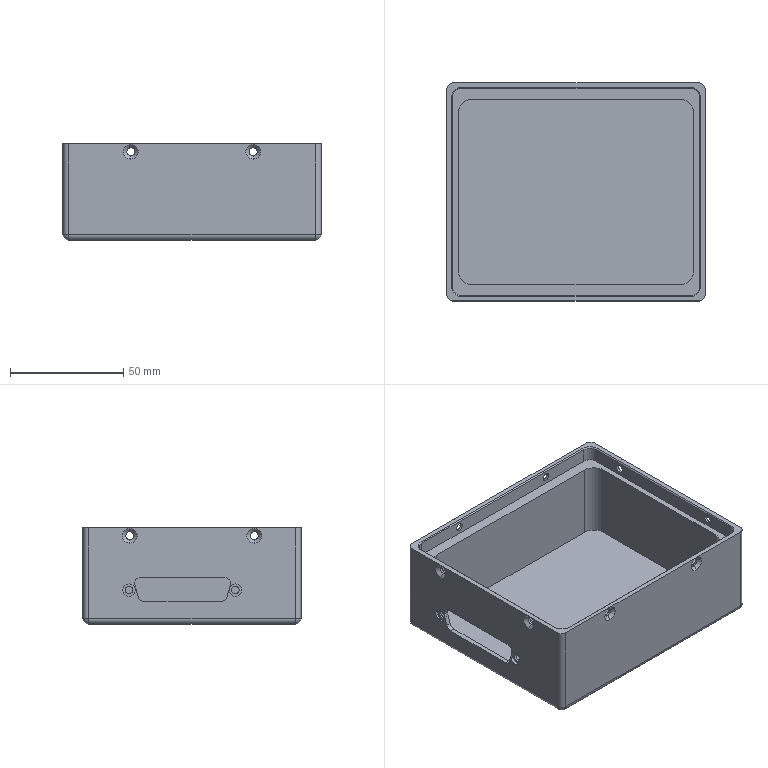Part | SolidWorks | features Cut 4, Fillet 4, 3DProfileFeature 3, HoleWzd 3, LPattern 3, MirrorPattern 2, Chamfer 1, Extrusion 1 | 1 solid | 100 faces | box 114 x 96.3 x 42.5 mm | volume 105828 mm3 | cylinder 45 | plane 31 | cone 20 | sphere 4 | commonest cylinder face diameters 3.5 x16 5 x13 3.3 x4 5.5 x4 8 x4 12 x4